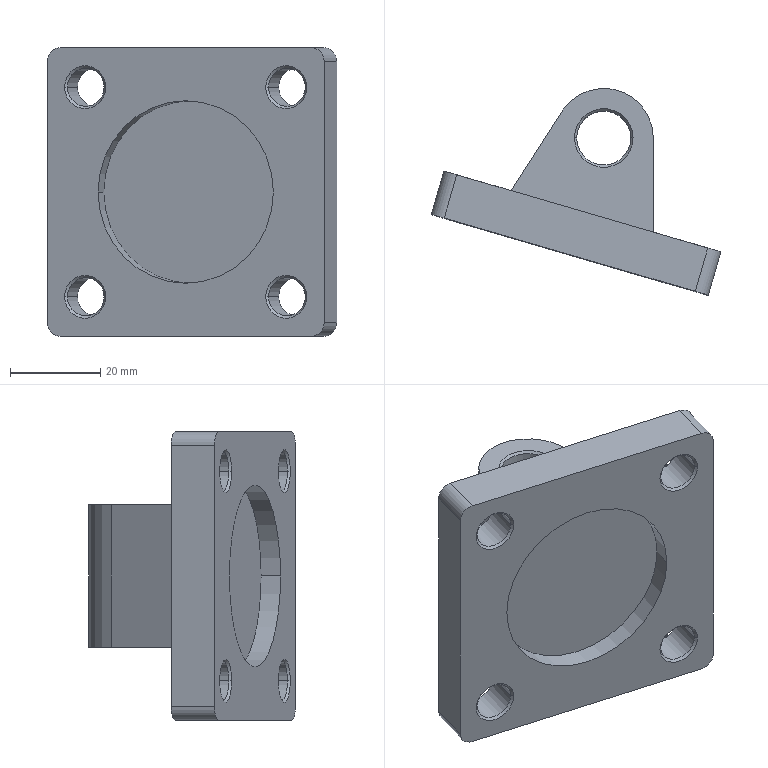Part | SolidWorks | features BaseBody 1 | 1 solid | 68 faces | box 64.24 x 45.879 x 64 mm | volume 49930 mm3 | cone 28 | cylinder 25 | plane 15 | commonest cylinder face diameters 8.5 x8 13.5 x8 6 x4 12 x2 40.5 x2 22 x1